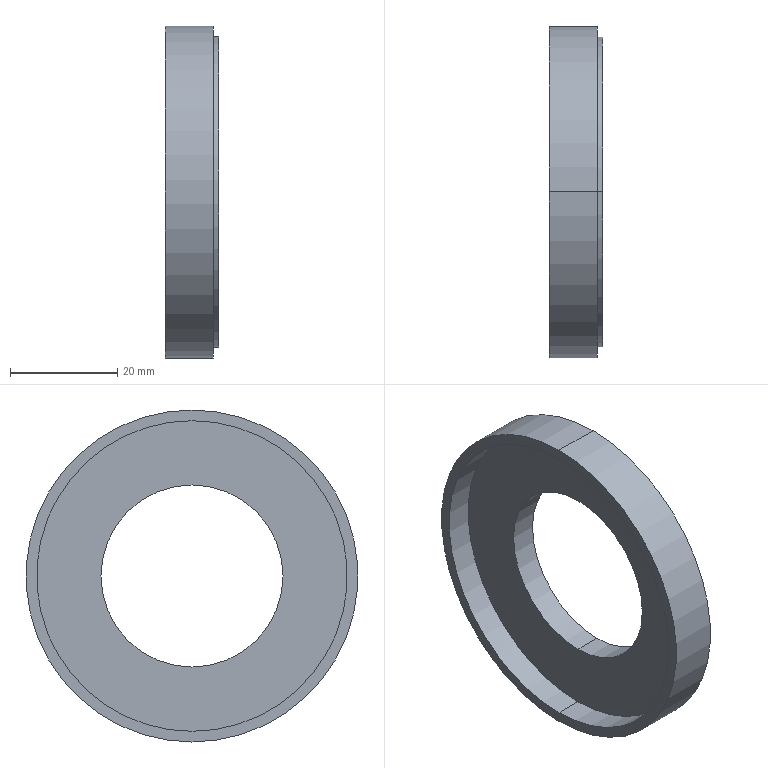Part | SolidWorks | features Revolution 1 | 1 solid | 12 faces | box 10 x 62 x 62 mm | volume 12064 mm3 | cylinder 8 | plane 4 | commonest cylinder face diameters 58 x4 34 x2 62 x2
STEP:
#1=CARTESIAN_POINT('',(-1.647,0.,-29.));
#2=VERTEX_POINT('',#1);
#3=CARTESIAN_POINT('',(-1.647,0.,29.));
#4=VERTEX_POINT('',#3);
#5=CARTESIAN_POINT('',(-1.647,0.,0.));
#6=DIRECTION('',(-1.,0.,0.));
#7=DIRECTION('',(0.,0.,1.));
#8=AXIS2_PLACEMENT_3D('',#5,#6,#7);
#9=CIRCLE('',#8,29.);
#10=EDGE_CURVE('',#2,#4,#9,.T.);
#11=ORIENTED_EDGE('',*,*,#10,.F.);
#12=CARTESIAN_POINT('',(-6.647,0.,-29.));
#13=VERTEX_POINT('',#12);
#14=CARTESIAN_POINT('',(0.,0.,-29.));
#15=DIRECTION('',(-1.,0.,0.));
#16=VECTOR('',#15,1000.);
#17=LINE('',#14,#16);
#18=EDGE_CURVE('',#2,#13,#17,.T.);
#19=ORIENTED_EDGE('',*,*,#18,.T.);
#20=CARTESIAN_POINT('',(-6.647,0.,29.));
#21=VERTEX_POINT('',#20);
#22=CARTESIAN_POINT('',(-6.647,0.,0.));
#23=DIRECTION('',(-1.,0.,0.));
#24=DIRECTION('',(0.,0.,1.));
#25=AXIS2_PLACEMENT_3D('',#22,#23,#24);
#26=CIRCLE('',#25,29.);
#27=EDGE_CURVE('',#13,#21,#26,.T.);
#28=ORIENTED_EDGE('',*,*,#27,.T.);
#29=CARTESIAN_POINT('',(0.,0.,29.));
#30=DIRECTION('',(-1.,0.,0.));
#31=VECTOR('',#30,1000.);
#32=LINE('',#29,#31);
#33=EDGE_CURVE('',#4,#21,#32,.T.);
#34=ORIENTED_EDGE('',*,*,#33,.F.);
#35=EDGE_LOOP('',(#11,#19,#28,#34));
#36=FACE_OUTER_BOUND('',#35,.T.);
#37=CARTESIAN_POINT('',(0.,0.,0.));
#38=DIRECTION('',(-1.,0.,0.));
#39=DIRECTION('',(0.,0.,1.));
#40=AXIS2_PLACEMENT_3D('',#37,#38,#39);
#41=CYLINDRICAL_SURFACE('',#40,29.);
#42=ADVANCED_FACE('',(#36),#41,.F.);
#43=CARTESIAN_POINT('',(2.353,0.,31.));
#44=VERTEX_POINT('',#43);
#45=CARTESIAN_POINT('',(2.353,0.,-31.));
#46=VERTEX_POINT('',#45);
#47=CARTESIAN_POINT('',(2.353,0.,0.));
#48=DIRECTION('',(-1.,0.,0.));
#49=DIRECTION('',(0.,0.,1.));
#50=AXIS2_PLACEMENT_3D('',#47,#48,#49);
#51=CIRCLE('',#50,31.);
#52=EDGE_CURVE('',#44,#46,#51,.T.);
#53=ORIENTED_EDGE('',*,*,#52,.T.);
#54=CARTESIAN_POINT('',(-6.647,0.,-31.));
#55=VERTEX_POINT('',#54);
#56=CARTESIAN_POINT('',(0.,0.,-31.));
#57=DIRECTION('',(-1.,0.,0.));
#58=VECTOR('',#57,1000.);
#59=LINE('',#56,#58);
#60=EDGE_CURVE('',#46,#55,#59,.T.);
#61=ORIENTED_EDGE('',*,*,#60,.T.);
#62=CARTESIAN_POINT('',(-6.647,0.,31.));
#63=VERTEX_POINT('',#62);
#64=CARTESIAN_POINT('',(-6.647,0.,0.));
#65=DIRECTION('',(-1.,0.,0.));
#66=DIRECTION('',(0.,0.,1.));
#67=AXIS2_PLACEMENT_3D('',#64,#65,#66);
#68=CIRCLE('',#67,31.);
#69=EDGE_CURVE('',#63,#55,#68,.T.);
#70=ORIENTED_EDGE('',*,*,#69,.F.);
#71=CARTESIAN_POINT('',(0.,0.,31.));
#72=DIRECTION('',(-1.,0.,0.));
#73=VECTOR('',#72,1000.);
#74=LINE('',#71,#73);
#75=EDGE_CURVE('',#44,#63,#74,.T.);
#76=ORIENTED_EDGE('',*,*,#75,.F.);
#77=EDGE_LOOP('',(#53,#61,#70,#76));
#78=FACE_OUTER_BOUND('',#77,.T.);
#79=CARTESIAN_POINT('',(0.,0.,0.));
#80=DIRECTION('',(-1.,0.,0.));
#81=DIRECTION('',(0.,0.,1.));
#82=AXIS2_PLACEMENT_3D('',#79,#80,#81);
#83=CYLINDRICAL_SURFACE('',#82,31.);
#84=ADVANCED_FACE('',(#78),#83,.T.);
#85=CARTESIAN_POINT('',(3.353,0.,29.));
#86=VERTEX_POINT('',#85);
#87=CARTESIAN_POINT('',(3.353,0.,-29.));
#88=VERTEX_POINT('',#87);
#89=CARTESIAN_POINT('',(3.353,0.,0.));
#90=DIRECTION('',(-1.,0.,0.));
#91=DIRECTION('',(0.,0.,1.));
#92=AXIS2_PLACEMENT_3D('',#89,#90,#91);
#93=CIRCLE('',#92,29.);
#94=EDGE_CURVE('',#86,#88,#93,.T.);
#95=ORIENTED_EDGE('',*,*,#94,.T.);
#96=CARTESIAN_POINT('',(2.353,0.,-29.));
#97=VERTEX_POINT('',#96);
#98=CARTESIAN_POINT('',(0.,0.,-29.));
#99=DIRECTION('',(-1.,0.,0.));
#100=VECTOR('',#99,1000.);
#101=LINE('',#98,#100);
#102=EDGE_CURVE('',#88,#97,#101,.T.);
#103=ORIENTED_EDGE('',*,*,#102,.T.);
#104=CARTESIAN_POINT('',(2.353,0.,29.));
#105=VERTEX_POINT('',#104);
#106=CARTESIAN_POINT('',(2.353,0.,0.));
#107=DIRECTION('',(-1.,0.,0.));
#108=DIRECTION('',(0.,0.,1.));
#109=AXIS2_PLACEMENT_3D('',#106,#107,#108);
#110=CIRCLE('',#109,29.);
#111=EDGE_CURVE('',#105,#97,#110,.T.);
#112=ORIENTED_EDGE('',*,*,#111,.F.);
#113=CARTESIAN_POINT('',(0.,0.,29.));
#114=DIRECTION('',(-1.,0.,0.));
#115=VECTOR('',#114,1000.);
#116=LINE('',#113,#115);
#117=EDGE_CURVE('',#86,#105,#116,.T.);
#118=ORIENTED_EDGE('',*,*,#117,.F.);
#119=EDGE_LOOP('',(#95,#103,#112,#118));
#120=FACE_OUTER_BOUND('',#119,.T.);
#121=CARTESIAN_POINT('',(0.,0.,0.));
#122=DIRECTION('',(-1.,0.,0.));
#123=DIRECTION('',(0.,0.,1.));
#124=AXIS2_PLACEMENT_3D('',#121,#122,#123);
#125=CYLINDRICAL_SURFACE('',#124,29.);
#126=ADVANCED_FACE('',(#120),#125,.T.);
#127=CARTESIAN_POINT('',(3.353,0.,-17.));
#128=VERTEX_POINT('',#127);
#129=CARTESIAN_POINT('',(3.353,0.,17.));
#130=VERTEX_POINT('',#129);
#131=CARTESIAN_POINT('',(3.353,0.,0.));
#132=DIRECTION('',(-1.,0.,0.));
#133=DIRECTION('',(0.,0.,1.));
#134=AXIS2_PLACEMENT_3D('',#131,#132,#133);
#135=CIRCLE('',#134,17.);
#136=EDGE_CURVE('',#128,#130,#135,.T.);
#137=ORIENTED_EDGE('',*,*,#136,.F.);
#138=CARTESIAN_POINT('',(-1.647,0.,-17.));
#139=VERTEX_POINT('',#138);
#140=CARTESIAN_POINT('',(0.,0.,-17.));
#141=DIRECTION('',(-1.,0.,0.));
#142=VECTOR('',#141,1000.);
#143=LINE('',#140,#142);
#144=EDGE_CURVE('',#128,#139,#143,.T.);
#145=ORIENTED_EDGE('',*,*,#144,.T.);
#146=CARTESIAN_POINT('',(-1.647,0.,17.));
#147=VERTEX_POINT('',#146);
#148=CARTESIAN_POINT('',(-1.647,0.,0.));
#149=DIRECTION('',(-1.,0.,0.));
#150=DIRECTION('',(0.,0.,1.));
#151=AXIS2_PLACEMENT_3D('',#148,#149,#150);
#152=CIRCLE('',#151,17.);
#153=EDGE_CURVE('',#139,#147,#152,.T.);
#154=ORIENTED_EDGE('',*,*,#153,.T.);
#155=CARTESIAN_POINT('',(0.,0.,17.));
#156=DIRECTION('',(-1.,0.,0.));
#157=VECTOR('',#156,1000.);
#158=LINE('',#155,#157);
#159=EDGE_CURVE('',#130,#147,#158,.T.);
#160=ORIENTED_EDGE('',*,*,#159,.F.);
#161=EDGE_LOOP('',(#137,#145,#154,#160));
#162=FACE_OUTER_BOUND('',#161,.T.);
#163=CARTESIAN_POINT('',(0.,0.,0.));
#164=DIRECTION('',(-1.,0.,0.));
#165=DIRECTION('',(0.,0.,1.));
#166=AXIS2_PLACEMENT_3D('',#163,#164,#165);
#167=CYLINDRICAL_SURFACE('',#166,17.);
#168=ADVANCED_FACE('',(#162),#167,.F.);
#169=CARTESIAN_POINT('',(-1.647,0.,0.));
#170=DIRECTION('',(-1.,0.,0.));
#171=DIRECTION('',(0.,0.,1.));
#172=AXIS2_PLACEMENT_3D('',#169,#170,#171);
#173=CIRCLE('',#172,17.);
#174=EDGE_CURVE('',#147,#139,#173,.T.);
#175=ORIENTED_EDGE('',*,*,#174,.F.);
#176=ORIENTED_EDGE('',*,*,#153,.F.);
#177=EDGE_LOOP('',(#175,#176));
#178=FACE_BOUND('',#177,.T.);
#179=CARTESIAN_POINT('',(-1.647,0.,0.));
#180=DIRECTION('',(-1.,0.,0.));
#181=DIRECTION('',(0.,0.,1.));
#182=AXIS2_PLACEMENT_3D('',#179,#180,#181);
#183=CIRCLE('',#182,29.);
#184=EDGE_CURVE('',#4,#2,#183,.T.);
#185=ORIENTED_EDGE('',*,*,#184,.T.);
#186=ORIENTED_EDGE('',*,*,#10,.T.);
#187=EDGE_LOOP('',(#185,#186));
#188=FACE_OUTER_BOUND('',#187,.T.);
#189=CARTESIAN_POINT('',(-1.647,29.,0.));
#190=DIRECTION('',(1.,0.,0.));
#191=DIRECTION('',(0.,0.,-1.));
#192=AXIS2_PLACEMENT_3D('',#189,#190,#191);
#193=PLANE('',#192);
#194=ADVANCED_FACE('',(#178,#188),#193,.F.);
#195=ORIENTED_EDGE('',*,*,#144,.F.);
#196=CARTESIAN_POINT('',(3.353,0.,0.));
#197=DIRECTION('',(-1.,0.,0.));
#198=DIRECTION('',(0.,0.,1.));
#199=AXIS2_PLACEMENT_3D('',#196,#197,#198);
#200=CIRCLE('',#199,17.);
#201=EDGE_CURVE('',#130,#128,#200,.T.);
#202=ORIENTED_EDGE('',*,*,#201,.F.);
#203=ORIENTED_EDGE('',*,*,#159,.T.);
#204=ORIENTED_EDGE('',*,*,#174,.T.);
#205=EDGE_LOOP('',(#195,#202,#203,#204));
#206=FACE_OUTER_BOUND('',#205,.T.);
#207=CARTESIAN_POINT('',(0.,0.,0.));
#208=DIRECTION('',(-1.,0.,0.));
#209=DIRECTION('',(0.,0.,1.));
#210=AXIS2_PLACEMENT_3D('',#207,#208,#209);
#211=CYLINDRICAL_SURFACE('',#210,17.);
#212=ADVANCED_FACE('',(#206),#211,.F.);
#213=ORIENTED_EDGE('',*,*,#94,.F.);
#214=CARTESIAN_POINT('',(3.353,0.,0.));
#215=DIRECTION('',(-1.,0.,0.));
#216=DIRECTION('',(0.,0.,1.));
#217=AXIS2_PLACEMENT_3D('',#214,#215,#216);
#218=CIRCLE('',#217,29.);
#219=EDGE_CURVE('',#88,#86,#218,.T.);
#220=ORIENTED_EDGE('',*,*,#219,.F.);
#221=EDGE_LOOP('',(#213,#220));
#222=FACE_OUTER_BOUND('',#221,.T.);
#223=ORIENTED_EDGE('',*,*,#201,.T.);
#224=ORIENTED_EDGE('',*,*,#136,.T.);
#225=EDGE_LOOP('',(#223,#224));
#226=FACE_BOUND('',#225,.T.);
#227=CARTESIAN_POINT('',(3.353,17.,0.));
#228=DIRECTION('',(-1.,0.,0.));
#229=DIRECTION('',(0.,0.,1.));
#230=AXIS2_PLACEMENT_3D('',#227,#228,#229);
#231=PLANE('',#230);
#232=ADVANCED_FACE('',(#222,#226),#231,.F.);
#233=ORIENTED_EDGE('',*,*,#102,.F.);
#234=ORIENTED_EDGE('',*,*,#219,.T.);
#235=ORIENTED_EDGE('',*,*,#117,.T.);
#236=CARTESIAN_POINT('',(2.353,0.,0.));
#237=DIRECTION('',(-1.,0.,0.));
#238=DIRECTION('',(0.,0.,1.));
#239=AXIS2_PLACEMENT_3D('',#236,#237,#238);
#240=CIRCLE('',#239,29.);
#241=EDGE_CURVE('',#97,#105,#240,.T.);
#242=ORIENTED_EDGE('',*,*,#241,.F.);
#243=EDGE_LOOP('',(#233,#234,#235,#242));
#244=FACE_OUTER_BOUND('',#243,.T.);
#245=CARTESIAN_POINT('',(0.,0.,0.));
#246=DIRECTION('',(-1.,0.,0.));
#247=DIRECTION('',(0.,0.,1.));
#248=AXIS2_PLACEMENT_3D('',#245,#246,#247);
#249=CYLINDRICAL_SURFACE('',#248,29.);
#250=ADVANCED_FACE('',(#244),#249,.T.);
#251=ORIENTED_EDGE('',*,*,#52,.F.);
#252=CARTESIAN_POINT('',(2.353,0.,0.));
#253=DIRECTION('',(-1.,0.,0.));
#254=DIRECTION('',(0.,0.,1.));
#255=AXIS2_PLACEMENT_3D('',#252,#253,#254);
#256=CIRCLE('',#255,31.);
#257=EDGE_CURVE('',#46,#44,#256,.T.);
#258=ORIENTED_EDGE('',*,*,#257,.F.);
#259=EDGE_LOOP('',(#251,#258));
#260=FACE_OUTER_BOUND('',#259,.T.);
#261=ORIENTED_EDGE('',*,*,#111,.T.);
#262=ORIENTED_EDGE('',*,*,#241,.T.);
#263=EDGE_LOOP('',(#261,#262));
#264=FACE_BOUND('',#263,.T.);
#265=CARTESIAN_POINT('',(2.353,29.,0.));
#266=DIRECTION('',(-1.,0.,0.));
#267=DIRECTION('',(0.,0.,1.));
#268=AXIS2_PLACEMENT_3D('',#265,#266,#267);
#269=PLANE('',#268);
#270=ADVANCED_FACE('',(#260,#264),#269,.F.);
#271=ORIENTED_EDGE('',*,*,#60,.F.);
#272=ORIENTED_EDGE('',*,*,#257,.T.);
#273=ORIENTED_EDGE('',*,*,#75,.T.);
#274=CARTESIAN_POINT('',(-6.647,0.,0.));
#275=DIRECTION('',(-1.,0.,0.));
#276=DIRECTION('',(0.,0.,1.));
#277=AXIS2_PLACEMENT_3D('',#274,#275,#276);
#278=CIRCLE('',#277,31.);
#279=EDGE_CURVE('',#55,#63,#278,.T.);
#280=ORIENTED_EDGE('',*,*,#279,.F.);
#281=EDGE_LOOP('',(#271,#272,#273,#280));
#282=FACE_OUTER_BOUND('',#281,.T.);
#283=CARTESIAN_POINT('',(0.,0.,0.));
#284=DIRECTION('',(-1.,0.,0.));
#285=DIRECTION('',(0.,0.,1.));
#286=AXIS2_PLACEMENT_3D('',#283,#284,#285);
#287=CYLINDRICAL_SURFACE('',#286,31.);
#288=ADVANCED_FACE('',(#282),#287,.T.);
#289=CARTESIAN_POINT('',(-6.647,0.,0.));
#290=DIRECTION('',(-1.,0.,0.));
#291=DIRECTION('',(0.,0.,1.));
#292=AXIS2_PLACEMENT_3D('',#289,#290,#291);
#293=CIRCLE('',#292,29.);
#294=EDGE_CURVE('',#21,#13,#293,.T.);
#295=ORIENTED_EDGE('',*,*,#294,.F.);
#296=ORIENTED_EDGE('',*,*,#27,.F.);
#297=EDGE_LOOP('',(#295,#296));
#298=FACE_BOUND('',#297,.T.);
#299=ORIENTED_EDGE('',*,*,#69,.T.);
#300=ORIENTED_EDGE('',*,*,#279,.T.);
#301=EDGE_LOOP('',(#299,#300));
#302=FACE_OUTER_BOUND('',#301,.T.);
#303=CARTESIAN_POINT('',(-6.647,31.,0.));
#304=DIRECTION('',(1.,0.,0.));
#305=DIRECTION('',(0.,0.,-1.));
#306=AXIS2_PLACEMENT_3D('',#303,#304,#305);
#307=PLANE('',#306);
#308=ADVANCED_FACE('',(#298,#302),#307,.F.);
#309=ORIENTED_EDGE('',*,*,#18,.F.);
#310=ORIENTED_EDGE('',*,*,#184,.F.);
#311=ORIENTED_EDGE('',*,*,#33,.T.);
#312=ORIENTED_EDGE('',*,*,#294,.T.);
#313=EDGE_LOOP('',(#309,#310,#311,#312));
#314=FACE_OUTER_BOUND('',#313,.T.);
#315=CARTESIAN_POINT('',(0.,0.,0.));
#316=DIRECTION('',(-1.,0.,0.));
#317=DIRECTION('',(0.,0.,1.));
#318=AXIS2_PLACEMENT_3D('',#315,#316,#317);
#319=CYLINDRICAL_SURFACE('',#318,29.);
#320=ADVANCED_FACE('',(#314),#319,.F.);
#321=CLOSED_SHELL('',(#42,#84,#126,#168,#194,#212,#232,#250,#270,#288,#308,#320));
#322=MANIFOLD_SOLID_BREP('',#321);
#323=CARTESIAN_POINT('',(0.,0.,0.));
#324=DIRECTION('',(0.,0.,1.));
#325=DIRECTION('',(1.,0.,0.));
#326=AXIS2_PLACEMENT_3D('',#323,#324,#325);
#327=(LENGTH_UNIT()NAMED_UNIT(*)SI_UNIT(.MILLI.,.METRE.));
#328=UNCERTAINTY_MEASURE_WITH_UNIT(LENGTH_MEASURE(0.00001),#327,'','');
#329=(NAMED_UNIT(*)PLANE_ANGLE_UNIT()SI_UNIT($,.RADIAN.));
#330=(NAMED_UNIT(*)SI_UNIT($,.STERADIAN.)SOLID_ANGLE_UNIT());
#331=(GEOMETRIC_REPRESENTATION_CONTEXT(3)GLOBAL_UNCERTAINTY_ASSIGNED_CONTEXT((#328))GLOBAL_UNIT_ASSIGNED_CONTEXT((#327,#329,#330))REPRESENTATION_CONTEXT('',''));
#332=ADVANCED_BREP_SHAPE_REPRESENTATION('',(#322,#326),#331);